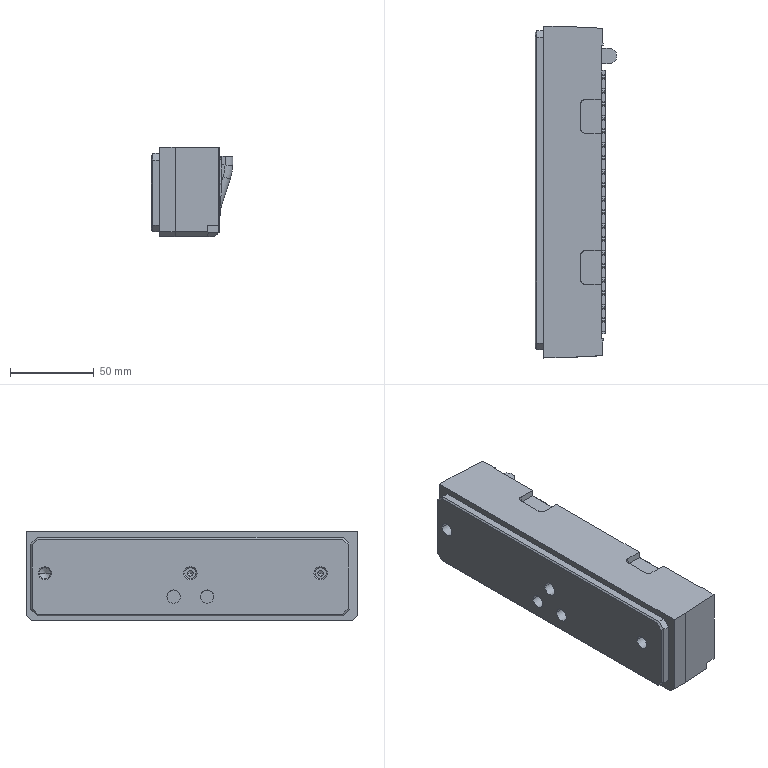Part | Creo | 1 solid | 1764 faces | box 48.993 x 198.6 x 53.738 mm | volume 391289 mm3 | spline 780 | plane 512 | cone 425 | cylinder 46 | torus 1 | commonest cylinder face diameters 8 x36 6 x4 2.01 x2 6.71 x2 9.045 x2